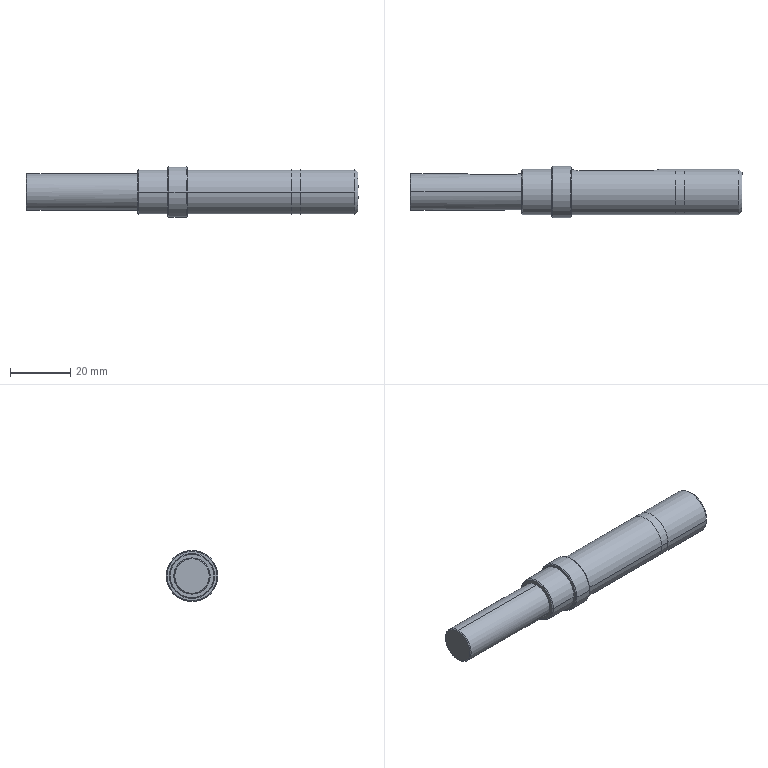Part | NX | 1 solid | 39 faces | box 110 x 17 x 17 mm | volume 16852 mm3 | cylinder 18 | plane 11 | cone 10 | commonest cylinder face diameters 15 x8 4 x3 5 x3 12 x2 17 x2